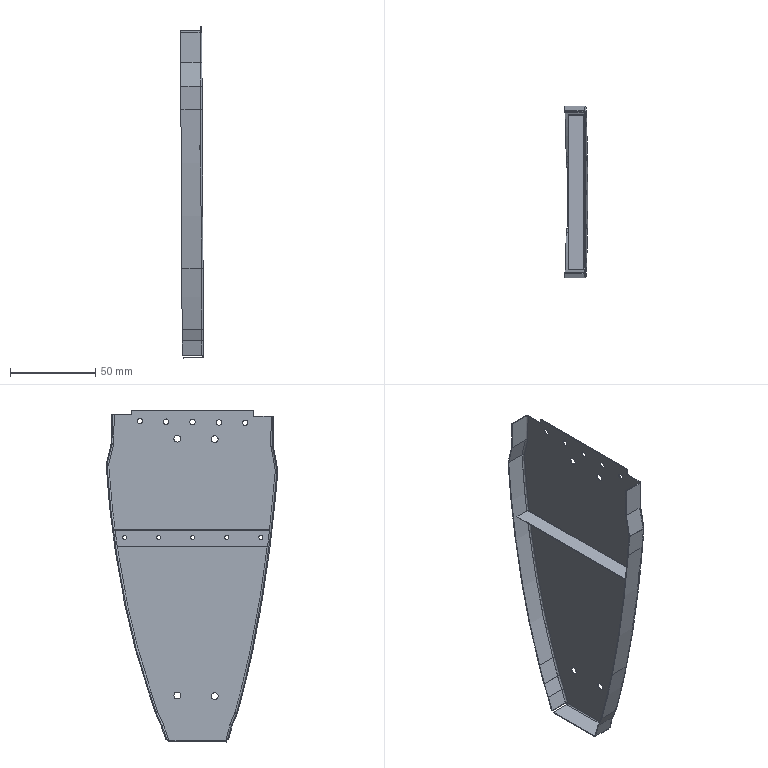Part | SolidWorks | features BaseBody 2 | 2 solids | 130 faces | box 13.553 x 101.015 x 195.172 mm | volume 11033 mm3 | cylinder 48 | spline 45 | plane 37 | commonest cylinder face diameters 2 x27 2.4 x10 4 x8 1 x3